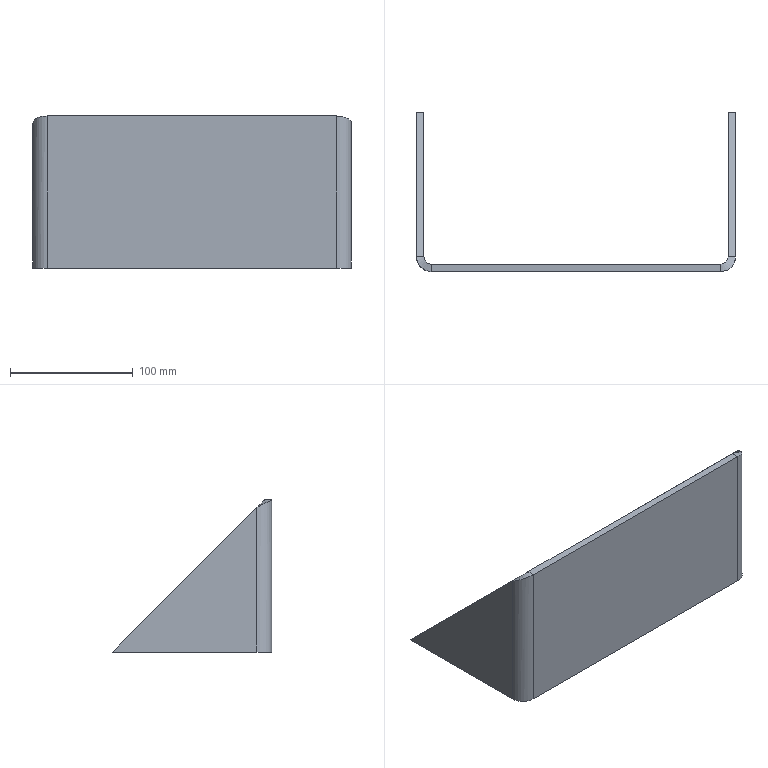Part | SolidWorks | features FlatPattern 1, ICE 1, SMBaseFlange 1, SheetMetal 1 | 1 solid | 20 faces | box 260 x 130 x 124 mm | volume 279794 mm3 | plane 14 | cylinder 4 | spline 2 | commonest cylinder face diameters 12 x2 24 x2
STEP:
#1=CARTESIAN_POINT('',(6.,130.,-62.));
#2=VERTEX_POINT('',#1);
#3=CARTESIAN_POINT('',(6.,12.,56.));
#4=VERTEX_POINT('',#3);
#5=CARTESIAN_POINT('',(6.,130.,-62.));
#6=DIRECTION('',(0.,-0.7071,0.7071));
#7=VECTOR('',#6,1000.);
#8=LINE('',#5,#7);
#9=EDGE_CURVE('',#2,#4,#8,.T.);
#10=ORIENTED_EDGE('',*,*,#9,.T.);
#11=CARTESIAN_POINT('',(6.,12.,-62.));
#12=VERTEX_POINT('',#11);
#13=CARTESIAN_POINT('',(6.,12.,62.));
#14=DIRECTION('',(0.,0.,-1.));
#15=VECTOR('',#14,1000.);
#16=LINE('',#13,#15);
#17=EDGE_CURVE('',#4,#12,#16,.T.);
#18=ORIENTED_EDGE('',*,*,#17,.T.);
#19=CARTESIAN_POINT('',(6.,0.,-62.));
#20=DIRECTION('',(0.,1.,0.));
#21=VECTOR('',#20,1000.);
#22=LINE('',#19,#21);
#23=EDGE_CURVE('',#12,#2,#22,.T.);
#24=ORIENTED_EDGE('',*,*,#23,.T.);
#25=EDGE_LOOP('',(#10,#18,#24));
#26=FACE_OUTER_BOUND('',#25,.T.);
#27=CARTESIAN_POINT('',(6.,0.,62.));
#28=DIRECTION('',(-1.,0.,0.));
#29=DIRECTION('',(0.,0.,1.));
#30=AXIS2_PLACEMENT_3D('',#27,#28,#29);
#31=PLANE('',#30);
#32=ADVANCED_FACE('',(#26),#31,.F.);
#33=CARTESIAN_POINT('',(0.,12.,56.));
#34=VERTEX_POINT('',#33);
#35=CARTESIAN_POINT('',(0.,12.,-62.));
#36=VERTEX_POINT('',#35);
#37=CARTESIAN_POINT('',(0.,12.,62.));
#38=DIRECTION('',(0.,0.,-1.));
#39=VECTOR('',#38,1000.);
#40=LINE('',#37,#39);
#41=EDGE_CURVE('',#34,#36,#40,.T.);
#42=ORIENTED_EDGE('',*,*,#41,.F.);
#43=CARTESIAN_POINT('',(0.,130.,-62.));
#44=VERTEX_POINT('',#43);
#45=CARTESIAN_POINT('',(0.,130.,-62.));
#46=DIRECTION('',(0.,-0.7071,0.7071));
#47=VECTOR('',#46,1000.);
#48=LINE('',#45,#47);
#49=EDGE_CURVE('',#44,#34,#48,.T.);
#50=ORIENTED_EDGE('',*,*,#49,.F.);
#51=CARTESIAN_POINT('',(0.,0.,-62.));
#52=DIRECTION('',(0.,1.,0.));
#53=VECTOR('',#52,1000.);
#54=LINE('',#51,#53);
#55=EDGE_CURVE('',#36,#44,#54,.T.);
#56=ORIENTED_EDGE('',*,*,#55,.F.);
#57=EDGE_LOOP('',(#42,#50,#56));
#58=FACE_OUTER_BOUND('',#57,.T.);
#59=CARTESIAN_POINT('',(0.,0.,62.));
#60=DIRECTION('',(-1.,0.,0.));
#61=DIRECTION('',(0.,0.,1.));
#62=AXIS2_PLACEMENT_3D('',#59,#60,#61);
#63=PLANE('',#62);
#64=ADVANCED_FACE('',(#58),#63,.T.);
#65=CARTESIAN_POINT('',(12.,0.,62.));
#66=VERTEX_POINT('',#65);
#67=CARTESIAN_POINT('',(12.,0.,-62.));
#68=VERTEX_POINT('',#67);
#69=CARTESIAN_POINT('',(12.,0.,62.));
#70=DIRECTION('',(0.,0.,-1.));
#71=VECTOR('',#70,1000.);
#72=LINE('',#69,#71);
#73=EDGE_CURVE('',#66,#68,#72,.T.);
#74=ORIENTED_EDGE('',*,*,#73,.F.);
#75=CARTESIAN_POINT('',(0.,12.,56.));
#76=CARTESIAN_POINT('',(0.,4.971,59.515));
#77=CARTESIAN_POINT('',(4.971,0.,62.));
#78=CARTESIAN_POINT('',(12.,0.,62.));
#79=(BOUNDED_CURVE()B_SPLINE_CURVE(3,(#75,#76,#77,#78),.UNSPECIFIED.,.F.,.T.)B_SPLINE_CURVE_WITH_KNOTS((4,4),(1.571,3.142),.UNSPECIFIED.)CURVE()GEOMETRIC_REPRESENTATION_ITEM()RATIONAL_B_SPLINE_CURVE((1.,0.8047,0.8047,1.))REPRESENTATION_ITEM(''));
#80=EDGE_CURVE('',#34,#66,#79,.T.);
#81=ORIENTED_EDGE('',*,*,#80,.F.);
#82=ORIENTED_EDGE('',*,*,#41,.T.);
#83=CARTESIAN_POINT('',(12.,12.,-62.));
#84=DIRECTION('',(0.,0.,-1.));
#85=DIRECTION('',(1.,0.,0.));
#86=AXIS2_PLACEMENT_3D('',#83,#84,#85);
#87=CIRCLE('',#86,12.);
#88=EDGE_CURVE('',#68,#36,#87,.T.);
#89=ORIENTED_EDGE('',*,*,#88,.F.);
#90=EDGE_LOOP('',(#74,#81,#82,#89));
#91=FACE_OUTER_BOUND('',#90,.T.);
#92=CARTESIAN_POINT('',(12.,12.,62.));
#93=DIRECTION('',(0.,0.,-1.));
#94=DIRECTION('',(-1.,0.,0.));
#95=AXIS2_PLACEMENT_3D('',#92,#93,#94);
#96=CYLINDRICAL_SURFACE('',#95,12.);
#97=ADVANCED_FACE('',(#91),#96,.T.);
#98=CARTESIAN_POINT('',(260.,12.,56.));
#99=VERTEX_POINT('',#98);
#100=CARTESIAN_POINT('',(260.,12.,-62.));
#101=VERTEX_POINT('',#100);
#102=CARTESIAN_POINT('',(260.,12.,62.));
#103=DIRECTION('',(0.,0.,-1.));
#104=VECTOR('',#103,1000.);
#105=LINE('',#102,#104);
#106=EDGE_CURVE('',#99,#101,#105,.T.);
#107=ORIENTED_EDGE('',*,*,#106,.F.);
#108=CARTESIAN_POINT('',(248.,0.,62.));
#109=VERTEX_POINT('',#108);
#110=CARTESIAN_POINT('',(248.,0.,62.));
#111=CARTESIAN_POINT('',(255.029,0.,62.));
#112=CARTESIAN_POINT('',(260.,4.971,59.515));
#113=CARTESIAN_POINT('',(260.,12.,56.));
#114=(BOUNDED_CURVE()B_SPLINE_CURVE(3,(#110,#111,#112,#113),.UNSPECIFIED.,.F.,.T.)B_SPLINE_CURVE_WITH_KNOTS((4,4),(3.142,4.712),.UNSPECIFIED.)CURVE()GEOMETRIC_REPRESENTATION_ITEM()RATIONAL_B_SPLINE_CURVE((1.,0.8047,0.8047,1.))REPRESENTATION_ITEM(''));
#115=EDGE_CURVE('',#109,#99,#114,.T.);
#116=ORIENTED_EDGE('',*,*,#115,.F.);
#117=CARTESIAN_POINT('',(248.,0.,-62.));
#118=VERTEX_POINT('',#117);
#119=CARTESIAN_POINT('',(248.,0.,62.));
#120=DIRECTION('',(0.,0.,-1.));
#121=VECTOR('',#120,1000.);
#122=LINE('',#119,#121);
#123=EDGE_CURVE('',#109,#118,#122,.T.);
#124=ORIENTED_EDGE('',*,*,#123,.T.);
#125=CARTESIAN_POINT('',(248.,12.,-62.));
#126=DIRECTION('',(0.,0.,-1.));
#127=DIRECTION('',(1.,0.,0.));
#128=AXIS2_PLACEMENT_3D('',#125,#126,#127);
#129=CIRCLE('',#128,12.);
#130=EDGE_CURVE('',#101,#118,#129,.T.);
#131=ORIENTED_EDGE('',*,*,#130,.F.);
#132=EDGE_LOOP('',(#107,#116,#124,#131));
#133=FACE_OUTER_BOUND('',#132,.T.);
#134=CARTESIAN_POINT('',(248.,12.,62.));
#135=DIRECTION('',(0.,0.,-1.));
#136=DIRECTION('',(-1.,0.,0.));
#137=AXIS2_PLACEMENT_3D('',#134,#135,#136);
#138=CYLINDRICAL_SURFACE('',#137,12.);
#139=ADVANCED_FACE('',(#133),#138,.T.);
#140=CARTESIAN_POINT('',(260.,130.,-62.));
#141=VERTEX_POINT('',#140);
#142=CARTESIAN_POINT('',(260.,0.,-62.));
#143=DIRECTION('',(0.,-1.,0.));
#144=VECTOR('',#143,1000.);
#145=LINE('',#142,#144);
#146=EDGE_CURVE('',#141,#101,#145,.T.);
#147=ORIENTED_EDGE('',*,*,#146,.F.);
#148=CARTESIAN_POINT('',(260.,3.,65.));
#149=DIRECTION('',(0.,0.7071,-0.7071));
#150=VECTOR('',#149,1000.);
#151=LINE('',#148,#150);
#152=EDGE_CURVE('',#99,#141,#151,.T.);
#153=ORIENTED_EDGE('',*,*,#152,.F.);
#154=ORIENTED_EDGE('',*,*,#106,.T.);
#155=EDGE_LOOP('',(#147,#153,#154));
#156=FACE_OUTER_BOUND('',#155,.T.);
#157=CARTESIAN_POINT('',(260.,0.,62.));
#158=DIRECTION('',(1.,0.,0.));
#159=DIRECTION('',(0.,0.,-1.));
#160=AXIS2_PLACEMENT_3D('',#157,#158,#159);
#161=PLANE('',#160);
#162=ADVANCED_FACE('',(#156),#161,.T.);
#163=CARTESIAN_POINT('',(254.,12.,56.));
#164=VERTEX_POINT('',#163);
#165=CARTESIAN_POINT('',(254.,130.,-62.));
#166=VERTEX_POINT('',#165);
#167=CARTESIAN_POINT('',(254.,3.,65.));
#168=DIRECTION('',(0.,0.7071,-0.7071));
#169=VECTOR('',#168,1000.);
#170=LINE('',#167,#169);
#171=EDGE_CURVE('',#164,#166,#170,.T.);
#172=ORIENTED_EDGE('',*,*,#171,.T.);
#173=CARTESIAN_POINT('',(254.,12.,-62.));
#174=VERTEX_POINT('',#173);
#175=CARTESIAN_POINT('',(254.,0.,-62.));
#176=DIRECTION('',(0.,-1.,0.));
#177=VECTOR('',#176,1000.);
#178=LINE('',#175,#177);
#179=EDGE_CURVE('',#166,#174,#178,.T.);
#180=ORIENTED_EDGE('',*,*,#179,.T.);
#181=CARTESIAN_POINT('',(254.,12.,62.));
#182=DIRECTION('',(0.,0.,-1.));
#183=VECTOR('',#182,1000.);
#184=LINE('',#181,#183);
#185=EDGE_CURVE('',#164,#174,#184,.T.);
#186=ORIENTED_EDGE('',*,*,#185,.F.);
#187=EDGE_LOOP('',(#172,#180,#186));
#188=FACE_OUTER_BOUND('',#187,.T.);
#189=CARTESIAN_POINT('',(254.,0.,62.));
#190=DIRECTION('',(1.,0.,0.));
#191=DIRECTION('',(0.,0.,-1.));
#192=AXIS2_PLACEMENT_3D('',#189,#190,#191);
#193=PLANE('',#192);
#194=ADVANCED_FACE('',(#188),#193,.F.);
#195=CARTESIAN_POINT('',(248.,6.,62.));
#196=VERTEX_POINT('',#195);
#197=CARTESIAN_POINT('',(248.,6.,62.));
#198=CARTESIAN_POINT('',(251.515,6.,62.));
#199=CARTESIAN_POINT('',(254.,8.485,59.515));
#200=CARTESIAN_POINT('',(254.,12.,56.));
#201=(BOUNDED_CURVE()B_SPLINE_CURVE(3,(#197,#198,#199,#200),.UNSPECIFIED.,.F.,.T.)B_SPLINE_CURVE_WITH_KNOTS((4,4),(3.142,4.712),.UNSPECIFIED.)CURVE()GEOMETRIC_REPRESENTATION_ITEM()RATIONAL_B_SPLINE_CURVE((1.,0.8047,0.8047,1.))REPRESENTATION_ITEM(''));
#202=EDGE_CURVE('',#196,#164,#201,.T.);
#203=ORIENTED_EDGE('',*,*,#202,.T.);
#204=ORIENTED_EDGE('',*,*,#185,.T.);
#205=CARTESIAN_POINT('',(248.,6.,-62.));
#206=VERTEX_POINT('',#205);
#207=CARTESIAN_POINT('',(248.,12.,-62.));
#208=DIRECTION('',(0.,0.,-1.));
#209=DIRECTION('',(1.,0.,0.));
#210=AXIS2_PLACEMENT_3D('',#207,#208,#209);
#211=CIRCLE('',#210,6.);
#212=EDGE_CURVE('',#174,#206,#211,.T.);
#213=ORIENTED_EDGE('',*,*,#212,.T.);
#214=CARTESIAN_POINT('',(248.,6.,62.));
#215=DIRECTION('',(0.,0.,-1.));
#216=VECTOR('',#215,1000.);
#217=LINE('',#214,#216);
#218=EDGE_CURVE('',#196,#206,#217,.T.);
#219=ORIENTED_EDGE('',*,*,#218,.F.);
#220=EDGE_LOOP('',(#203,#204,#213,#219));
#221=FACE_OUTER_BOUND('',#220,.T.);
#222=CARTESIAN_POINT('',(248.,12.,62.));
#223=DIRECTION('',(0.,0.,-1.));
#224=DIRECTION('',(-1.,0.,0.));
#225=AXIS2_PLACEMENT_3D('',#222,#223,#224);
#226=CYLINDRICAL_SURFACE('',#225,6.);
#227=ADVANCED_FACE('',(#221),#226,.F.);
#228=CARTESIAN_POINT('',(12.,6.,62.));
#229=VERTEX_POINT('',#228);
#230=CARTESIAN_POINT('',(6.,12.,56.));
#231=CARTESIAN_POINT('',(6.,8.485,59.515));
#232=CARTESIAN_POINT('',(8.485,6.,62.));
#233=CARTESIAN_POINT('',(12.,6.,62.));
#234=(BOUNDED_CURVE()B_SPLINE_CURVE(3,(#230,#231,#232,#233),.UNSPECIFIED.,.F.,.T.)B_SPLINE_CURVE_WITH_KNOTS((4,4),(1.571,3.142),.UNSPECIFIED.)CURVE()GEOMETRIC_REPRESENTATION_ITEM()RATIONAL_B_SPLINE_CURVE((1.,0.8047,0.8047,1.))REPRESENTATION_ITEM(''));
#235=EDGE_CURVE('',#4,#229,#234,.T.);
#236=ORIENTED_EDGE('',*,*,#235,.T.);
#237=CARTESIAN_POINT('',(12.,6.,-62.));
#238=VERTEX_POINT('',#237);
#239=CARTESIAN_POINT('',(12.,6.,62.));
#240=DIRECTION('',(0.,0.,-1.));
#241=VECTOR('',#240,1000.);
#242=LINE('',#239,#241);
#243=EDGE_CURVE('',#229,#238,#242,.T.);
#244=ORIENTED_EDGE('',*,*,#243,.T.);
#245=CARTESIAN_POINT('',(12.,12.,-62.));
#246=DIRECTION('',(0.,0.,-1.));
#247=DIRECTION('',(1.,0.,0.));
#248=AXIS2_PLACEMENT_3D('',#245,#246,#247);
#249=CIRCLE('',#248,6.);
#250=EDGE_CURVE('',#238,#12,#249,.T.);
#251=ORIENTED_EDGE('',*,*,#250,.T.);
#252=ORIENTED_EDGE('',*,*,#17,.F.);
#253=EDGE_LOOP('',(#236,#244,#251,#252));
#254=FACE_OUTER_BOUND('',#253,.T.);
#255=CARTESIAN_POINT('',(12.,12.,62.));
#256=DIRECTION('',(0.,0.,-1.));
#257=DIRECTION('',(-1.,0.,0.));
#258=AXIS2_PLACEMENT_3D('',#255,#256,#257);
#259=CYLINDRICAL_SURFACE('',#258,6.);
#260=ADVANCED_FACE('',(#254),#259,.F.);
#261=CARTESIAN_POINT('',(0.,0.,62.));
#262=DIRECTION('',(-1.,0.,0.));
#263=VECTOR('',#262,1000.);
#264=LINE('',#261,#263);
#265=EDGE_CURVE('',#109,#66,#264,.T.);
#266=ORIENTED_EDGE('',*,*,#265,.F.);
#267=CARTESIAN_POINT('',(248.,0.,62.));
#268=DIRECTION('',(0.,1.,0.));
#269=VECTOR('',#268,1000.);
#270=LINE('',#267,#269);
#271=EDGE_CURVE('',#109,#196,#270,.T.);
#272=ORIENTED_EDGE('',*,*,#271,.T.);
#273=CARTESIAN_POINT('',(0.,6.,62.));
#274=DIRECTION('',(-1.,0.,0.));
#275=VECTOR('',#274,1000.);
#276=LINE('',#273,#275);
#277=EDGE_CURVE('',#196,#229,#276,.T.);
#278=ORIENTED_EDGE('',*,*,#277,.T.);
#279=CARTESIAN_POINT('',(12.,6.,62.));
#280=DIRECTION('',(0.,-1.,0.));
#281=VECTOR('',#280,1000.);
#282=LINE('',#279,#281);
#283=EDGE_CURVE('',#229,#66,#282,.T.);
#284=ORIENTED_EDGE('',*,*,#283,.T.);
#285=EDGE_LOOP('',(#266,#272,#278,#284));
#286=FACE_OUTER_BOUND('',#285,.T.);
#287=CARTESIAN_POINT('',(254.,12.,62.));
#288=DIRECTION('',(0.,0.,1.));
#289=DIRECTION('',(1.,0.,0.));
#290=AXIS2_PLACEMENT_3D('',#287,#288,#289);
#291=PLANE('',#290);
#292=ADVANCED_FACE('',(#286),#291,.T.);
#293=CARTESIAN_POINT('',(260.,12.,-62.));
#294=DIRECTION('',(-1.,0.,0.));
#295=VECTOR('',#294,1000.);
#296=LINE('',#293,#295);
#297=EDGE_CURVE('',#101,#174,#296,.T.);
#298=ORIENTED_EDGE('',*,*,#297,.F.);
#299=ORIENTED_EDGE('',*,*,#130,.T.);
#300=CARTESIAN_POINT('',(248.,6.,-62.));
#301=DIRECTION('',(0.,-1.,0.));
#302=VECTOR('',#301,1000.);
#303=LINE('',#300,#302);
#304=EDGE_CURVE('',#206,#118,#303,.T.);
#305=ORIENTED_EDGE('',*,*,#304,.F.);
#306=ORIENTED_EDGE('',*,*,#212,.F.);
#307=EDGE_LOOP('',(#298,#299,#305,#306));
#308=FACE_OUTER_BOUND('',#307,.T.);
#309=CARTESIAN_POINT('',(260.,12.,-62.));
#310=DIRECTION('',(0.,0.,-1.));
#311=DIRECTION('',(-1.,0.,0.));
#312=AXIS2_PLACEMENT_3D('',#309,#310,#311);
#313=PLANE('',#312);
#314=ADVANCED_FACE('',(#308),#313,.T.);
#315=ORIENTED_EDGE('',*,*,#146,.T.);
#316=ORIENTED_EDGE('',*,*,#297,.T.);
#317=ORIENTED_EDGE('',*,*,#179,.F.);
#318=CARTESIAN_POINT('',(254.,130.,-62.));
#319=DIRECTION('',(1.,0.,0.));
#320=VECTOR('',#319,1000.);
#321=LINE('',#318,#320);
#322=EDGE_CURVE('',#166,#141,#321,.T.);
#323=ORIENTED_EDGE('',*,*,#322,.T.);
#324=EDGE_LOOP('',(#315,#316,#317,#323));
#325=FACE_OUTER_BOUND('',#324,.T.);
#326=CARTESIAN_POINT('',(248.,6.,-62.));
#327=DIRECTION('',(0.,0.,-1.));
#328=DIRECTION('',(-1.,0.,0.));
#329=AXIS2_PLACEMENT_3D('',#326,#327,#328);
#330=PLANE('',#329);
#331=ADVANCED_FACE('',(#325),#330,.T.);
#332=CARTESIAN_POINT('',(12.,0.,-62.));
#333=DIRECTION('',(0.,1.,0.));
#334=VECTOR('',#333,1000.);
#335=LINE('',#332,#334);
#336=EDGE_CURVE('',#68,#238,#335,.T.);
#337=ORIENTED_EDGE('',*,*,#336,.F.);
#338=ORIENTED_EDGE('',*,*,#88,.T.);
#339=CARTESIAN_POINT('',(6.,12.,-62.));
#340=DIRECTION('',(-1.,0.,0.));
#341=VECTOR('',#340,1000.);
#342=LINE('',#339,#341);
#343=EDGE_CURVE('',#12,#36,#342,.T.);
#344=ORIENTED_EDGE('',*,*,#343,.F.);
#345=ORIENTED_EDGE('',*,*,#250,.F.);
#346=EDGE_LOOP('',(#337,#338,#344,#345));
#347=FACE_OUTER_BOUND('',#346,.T.);
#348=CARTESIAN_POINT('',(12.,0.,-62.));
#349=DIRECTION('',(0.,0.,-1.));
#350=DIRECTION('',(-1.,0.,0.));
#351=AXIS2_PLACEMENT_3D('',#348,#349,#350);
#352=PLANE('',#351);
#353=ADVANCED_FACE('',(#347),#352,.T.);
#354=CARTESIAN_POINT('',(0.,0.,-62.));
#355=DIRECTION('',(-1.,0.,0.));
#356=VECTOR('',#355,1000.);
#357=LINE('',#354,#356);
#358=EDGE_CURVE('',#118,#68,#357,.T.);
#359=ORIENTED_EDGE('',*,*,#358,.T.);
#360=ORIENTED_EDGE('',*,*,#336,.T.);
#361=CARTESIAN_POINT('',(0.,6.,-62.));
#362=DIRECTION('',(-1.,0.,0.));
#363=VECTOR('',#362,1000.);
#364=LINE('',#361,#363);
#365=EDGE_CURVE('',#206,#238,#364,.T.);
#366=ORIENTED_EDGE('',*,*,#365,.F.);
#367=ORIENTED_EDGE('',*,*,#304,.T.);
#368=EDGE_LOOP('',(#359,#360,#366,#367));
#369=FACE_OUTER_BOUND('',#368,.T.);
#370=CARTESIAN_POINT('',(6.,12.,-62.));
#371=DIRECTION('',(0.,0.,-1.));
#372=DIRECTION('',(-1.,0.,0.));
#373=AXIS2_PLACEMENT_3D('',#370,#371,#372);
#374=PLANE('',#373);
#375=ADVANCED_FACE('',(#369),#374,.T.);
#376=ORIENTED_EDGE('',*,*,#358,.F.);
#377=ORIENTED_EDGE('',*,*,#123,.F.);
#378=ORIENTED_EDGE('',*,*,#265,.T.);
#379=ORIENTED_EDGE('',*,*,#73,.T.);
#380=EDGE_LOOP('',(#376,#377,#378,#379));
#381=FACE_OUTER_BOUND('',#380,.T.);
#382=CARTESIAN_POINT('',(0.,0.,62.));
#383=DIRECTION('',(0.,-1.,0.));
#384=DIRECTION('',(0.,0.,-1.));
#385=AXIS2_PLACEMENT_3D('',#382,#383,#384);
#386=PLANE('',#385);
#387=ADVANCED_FACE('',(#381),#386,.T.);
#388=ORIENTED_EDGE('',*,*,#365,.T.);
#389=ORIENTED_EDGE('',*,*,#243,.F.);
#390=ORIENTED_EDGE('',*,*,#277,.F.);
#391=ORIENTED_EDGE('',*,*,#218,.T.);
#392=EDGE_LOOP('',(#388,#389,#390,#391));
#393=FACE_OUTER_BOUND('',#392,.T.);
#394=CARTESIAN_POINT('',(0.,6.,62.));
#395=DIRECTION('',(0.,-1.,0.));
#396=DIRECTION('',(0.,0.,-1.));
#397=AXIS2_PLACEMENT_3D('',#394,#395,#396);
#398=PLANE('',#397);
#399=ADVANCED_FACE('',(#393),#398,.F.);
#400=ORIENTED_EDGE('',*,*,#23,.F.);
#401=ORIENTED_EDGE('',*,*,#343,.T.);
#402=ORIENTED_EDGE('',*,*,#55,.T.);
#403=CARTESIAN_POINT('',(0.,130.,-62.));
#404=DIRECTION('',(1.,0.,0.));
#405=VECTOR('',#404,1000.);
#406=LINE('',#403,#405);
#407=EDGE_CURVE('',#44,#2,#406,.T.);
#408=ORIENTED_EDGE('',*,*,#407,.T.);
#409=EDGE_LOOP('',(#400,#401,#402,#408));
#410=FACE_OUTER_BOUND('',#409,.T.);
#411=CARTESIAN_POINT('',(12.,12.,-62.));
#412=DIRECTION('',(0.,0.,1.));
#413=DIRECTION('',(1.,0.,0.));
#414=AXIS2_PLACEMENT_3D('',#411,#412,#413);
#415=PLANE('',#414);
#416=ADVANCED_FACE('',(#410),#415,.F.);
#417=ORIENTED_EDGE('',*,*,#49,.T.);
#418=CARTESIAN_POINT('',(0.,12.,56.));
#419=DIRECTION('',(1.,0.,0.));
#420=VECTOR('',#419,1000.);
#421=LINE('',#418,#420);
#422=EDGE_CURVE('',#34,#4,#421,.T.);
#423=ORIENTED_EDGE('',*,*,#422,.T.);
#424=ORIENTED_EDGE('',*,*,#9,.F.);
#425=ORIENTED_EDGE('',*,*,#407,.F.);
#426=EDGE_LOOP('',(#417,#423,#424,#425));
#427=FACE_OUTER_BOUND('',#426,.T.);
#428=CARTESIAN_POINT('',(0.,130.,-62.));
#429=DIRECTION('',(0.,-0.7071,-0.7071));
#430=DIRECTION('',(0.,-0.7071,0.7071));
#431=AXIS2_PLACEMENT_3D('',#428,#429,#430);
#432=PLANE('',#431);
#433=ADVANCED_FACE('',(#427),#432,.F.);
#434=ORIENTED_EDGE('',*,*,#283,.F.);
#435=ORIENTED_EDGE('',*,*,#235,.F.);
#436=ORIENTED_EDGE('',*,*,#422,.F.);
#437=ORIENTED_EDGE('',*,*,#80,.T.);
#438=EDGE_LOOP('',(#434,#435,#436,#437));
#439=FACE_OUTER_BOUND('',#438,.T.);
#440=CARTESIAN_POINT('',(12.,24.,50.));
#441=CARTESIAN_POINT('',(12.,22.,50.));
#442=CARTESIAN_POINT('',(12.,20.,50.));
#443=CARTESIAN_POINT('',(12.,18.,50.));
#444=CARTESIAN_POINT('',(-12.,24.,50.));
#445=CARTESIAN_POINT('',(-8.,22.,50.));
#446=CARTESIAN_POINT('',(-4.,20.,50.));
#447=CARTESIAN_POINT('',(0.,18.,50.));
#448=CARTESIAN_POINT('',(-12.,0.,62.));
#449=CARTESIAN_POINT('',(-8.,2.,62.));
#450=CARTESIAN_POINT('',(-4.,4.,62.));
#451=CARTESIAN_POINT('',(0.,6.,62.));
#452=CARTESIAN_POINT('',(12.,0.,62.));
#453=CARTESIAN_POINT('',(12.,2.,62.));
#454=CARTESIAN_POINT('',(12.,4.,62.));
#455=CARTESIAN_POINT('',(12.,6.,62.));
#456=CARTESIAN_POINT('',(36.,0.,62.));
#457=CARTESIAN_POINT('',(32.,2.,62.));
#458=CARTESIAN_POINT('',(28.,4.,62.));
#459=CARTESIAN_POINT('',(24.,6.,62.));
#460=CARTESIAN_POINT('',(36.,24.,50.));
#461=CARTESIAN_POINT('',(32.,22.,50.));
#462=CARTESIAN_POINT('',(28.,20.,50.));
#463=CARTESIAN_POINT('',(24.,18.,50.));
#464=CARTESIAN_POINT('',(12.,24.,50.));
#465=CARTESIAN_POINT('',(12.,22.,50.));
#466=CARTESIAN_POINT('',(12.,20.,50.));
#467=CARTESIAN_POINT('',(12.,18.,50.));
#468=(BOUNDED_SURFACE()B_SPLINE_SURFACE(3,3,((#440,#441,#442,#443),(#444,#445,#446,#447),(#448,#449,#450,#451),(#452,#453,#454,#455),(#456,#457,#458,#459),(#460,#461,#462,#463),(#464,#465,#466,#467)),.UNSPECIFIED.,.T.,.F.,.F.)B_SPLINE_SURFACE_WITH_KNOTS((4,3,4),(4,4),(0.,0.5,1.),(0.,1.),.UNSPECIFIED.)GEOMETRIC_REPRESENTATION_ITEM()RATIONAL_B_SPLINE_SURFACE(((1.,1.,1.,1.),(0.3333,0.3333,0.3333,0.3333),(0.3333,0.3333,0.3333,0.3333),(1.,1.,1.,1.),(0.3333,0.3333,0.3333,0.3333),(0.3333,0.3333,0.3333,0.3333),(1.,1.,1.,1.)))REPRESENTATION_ITEM('')SURFACE());
#469=ADVANCED_FACE('',(#439),#468,.T.);
#470=ORIENTED_EDGE('',*,*,#322,.F.);
#471=ORIENTED_EDGE('',*,*,#171,.F.);
#472=CARTESIAN_POINT('',(254.,12.,56.));
#473=DIRECTION('',(1.,0.,0.));
#474=VECTOR('',#473,1000.);
#475=LINE('',#472,#474);
#476=EDGE_CURVE('',#164,#99,#475,.T.);
#477=ORIENTED_EDGE('',*,*,#476,.T.);
#478=ORIENTED_EDGE('',*,*,#152,.T.);
#479=EDGE_LOOP('',(#470,#471,#477,#478));
#480=FACE_OUTER_BOUND('',#479,.T.);
#481=CARTESIAN_POINT('',(254.,3.,65.));
#482=DIRECTION('',(0.,-0.7071,-0.7071));
#483=DIRECTION('',(0.,0.7071,-0.7071));
#484=AXIS2_PLACEMENT_3D('',#481,#482,#483);
#485=PLANE('',#484);
#486=ADVANCED_FACE('',(#480),#485,.F.);
#487=ORIENTED_EDGE('',*,*,#476,.F.);
#488=ORIENTED_EDGE('',*,*,#202,.F.);
#489=ORIENTED_EDGE('',*,*,#271,.F.);
#490=ORIENTED_EDGE('',*,*,#115,.T.);
#491=EDGE_LOOP('',(#487,#488,#489,#490));
#492=FACE_OUTER_BOUND('',#491,.T.);
#493=CARTESIAN_POINT('',(248.,24.,50.));
#494=CARTESIAN_POINT('',(248.,22.,50.));
#495=CARTESIAN_POINT('',(248.,20.,50.));
#496=CARTESIAN_POINT('',(248.,18.,50.));
#497=CARTESIAN_POINT('',(224.,24.,50.));
#498=CARTESIAN_POINT('',(228.,22.,50.));
#499=CARTESIAN_POINT('',(232.,20.,50.));
#500=CARTESIAN_POINT('',(236.,18.,50.));
#501=CARTESIAN_POINT('',(224.,0.,62.));
#502=CARTESIAN_POINT('',(228.,2.,62.));
#503=CARTESIAN_POINT('',(232.,4.,62.));
#504=CARTESIAN_POINT('',(236.,6.,62.));
#505=CARTESIAN_POINT('',(248.,0.,62.));
#506=CARTESIAN_POINT('',(248.,2.,62.));
#507=CARTESIAN_POINT('',(248.,4.,62.));
#508=CARTESIAN_POINT('',(248.,6.,62.));
#509=CARTESIAN_POINT('',(272.,0.,62.));
#510=CARTESIAN_POINT('',(268.,2.,62.));
#511=CARTESIAN_POINT('',(264.,4.,62.));
#512=CARTESIAN_POINT('',(260.,6.,62.));
#513=CARTESIAN_POINT('',(272.,24.,50.));
#514=CARTESIAN_POINT('',(268.,22.,50.));
#515=CARTESIAN_POINT('',(264.,20.,50.));
#516=CARTESIAN_POINT('',(260.,18.,50.));
#517=CARTESIAN_POINT('',(248.,24.,50.));
#518=CARTESIAN_POINT('',(248.,22.,50.));
#519=CARTESIAN_POINT('',(248.,20.,50.));
#520=CARTESIAN_POINT('',(248.,18.,50.));
#521=(BOUNDED_SURFACE()B_SPLINE_SURFACE(3,3,((#493,#494,#495,#496),(#497,#498,#499,#500),(#501,#502,#503,#504),(#505,#506,#507,#508),(#509,#510,#511,#512),(#513,#514,#515,#516),(#517,#518,#519,#520)),.UNSPECIFIED.,.T.,.F.,.T.)B_SPLINE_SURFACE_WITH_KNOTS((4,3,4),(4,4),(0.,0.5,1.),(0.,1.),.UNSPECIFIED.)GEOMETRIC_REPRESENTATION_ITEM()RATIONAL_B_SPLINE_SURFACE(((1.,1.,1.,1.),(0.3333,0.3333,0.3333,0.3333),(0.3333,0.3333,0.3333,0.3333),(1.,1.,1.,1.),(0.3333,0.3333,0.3333,0.3333),(0.3333,0.3333,0.3333,0.3333),(1.,1.,1.,1.)))REPRESENTATION_ITEM('')SURFACE());
#522=ADVANCED_FACE('',(#492),#521,.T.);
#523=CLOSED_SHELL('',(#32,#64,#97,#139,#162,#194,#227,#260,#292,#314,#331,#353,#375,#387,#399,#416,#433,#469,#486,#522));
#524=MANIFOLD_SOLID_BREP('',#523);
#525=CARTESIAN_POINT('',(0.,0.,0.));
#526=DIRECTION('',(0.,0.,1.));
#527=DIRECTION('',(1.,0.,0.));
#528=AXIS2_PLACEMENT_3D('',#525,#526,#527);
#529=(LENGTH_UNIT()NAMED_UNIT(*)SI_UNIT(.MILLI.,.METRE.));
#530=UNCERTAINTY_MEASURE_WITH_UNIT(LENGTH_MEASURE(0.00001),#529,'','');
#531=(NAMED_UNIT(*)PLANE_ANGLE_UNIT()SI_UNIT($,.RADIAN.));
#532=(NAMED_UNIT(*)SI_UNIT($,.STERADIAN.)SOLID_ANGLE_UNIT());
#533=(GEOMETRIC_REPRESENTATION_CONTEXT(3)GLOBAL_UNCERTAINTY_ASSIGNED_CONTEXT((#530))GLOBAL_UNIT_ASSIGNED_CONTEXT((#529,#531,#532))REPRESENTATION_CONTEXT('',''));
#534=ADVANCED_BREP_SHAPE_REPRESENTATION('',(#524,#528),#533);